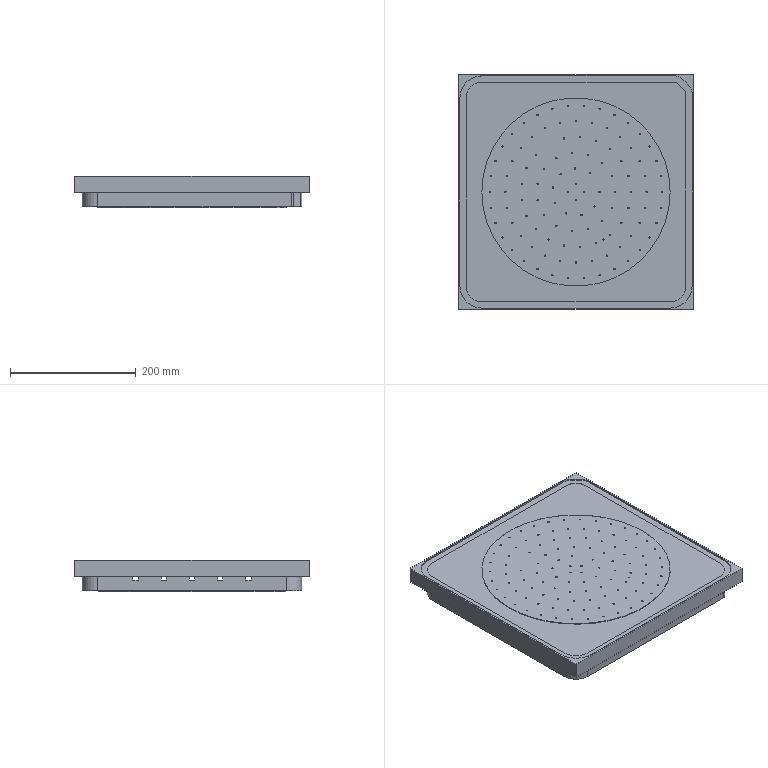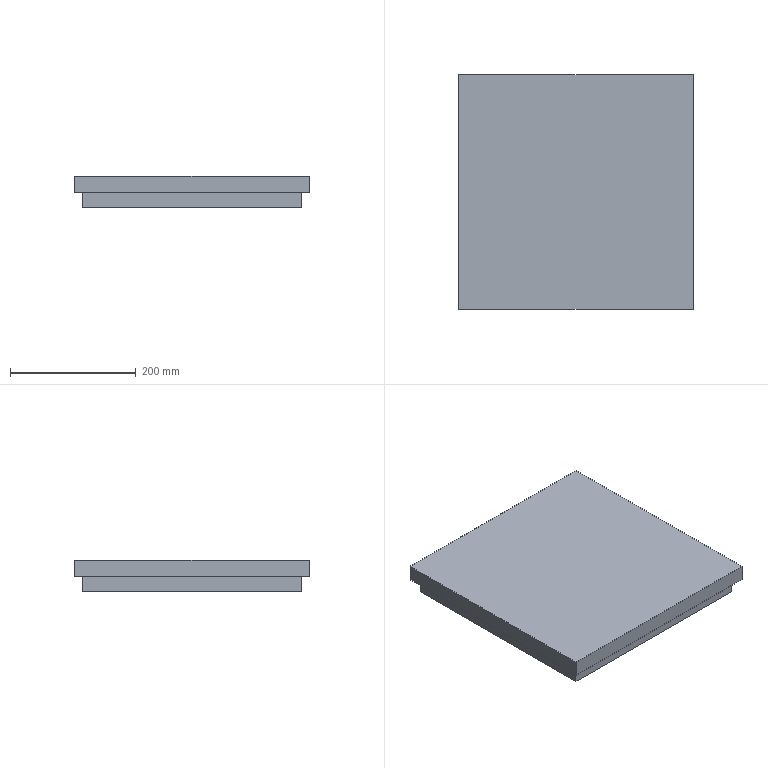CAM job | NX | 3-axis milling, drilling | part box 374 x 374 x 49.5 mm | stock box 374 x 374 x 49.5 mm
Tools:
number,name,description,diameter,corner_radius,flute_length,length,flutes
0,V2.0,Drilling Tool,2.0,0.0,35.0,50.0,2
0,D10,No Description,10.0,0.0,20.0,60.0,2
0,D8,No Description,8.0,0.0,0.0,40.0,2
0,D16R0.8,No Description,16.0,0.8,50.0,90.0,2
Operations:
program,operation,operation_type,tool,method,geometry_group,spindle_rpm,surface_speed,feed_per_tooth,feed_cut,feed_plunge,cut_length_mm,path_length_mm,cut_time_min,machine_time_min
B-1,01,CavityMilling,D16R0.8,METHOD,22B,7000.0,1099.0,0.3214,4500.0,100.0,75108.867,76038.412,16.691,16.784
B-2,02,Operation,V2.0,METHOD,22B,2000.0,75.0,0.0375,150.0,0.0,555.0,4398.211,3.7,4.084
B-3,03,FaceMilling,D10,METHOD,22B,7000.0,1099.0,0.2857,4000.0,100.0,21337.5,21825.412,5.334,5.383
B-3,003,PlanarMilling,D10,METHOD,22B,7000.0,571.0,0.2857,4000.0,100.0,28663.803,28849.603,7.166,7.184
C-1,CAVITY_MILL_1,CavityMilling,D8,METHOD,23C,7000.0,1099.0,0.3214,4500.0,100.0,171627.965,172384.855,38.139,38.215